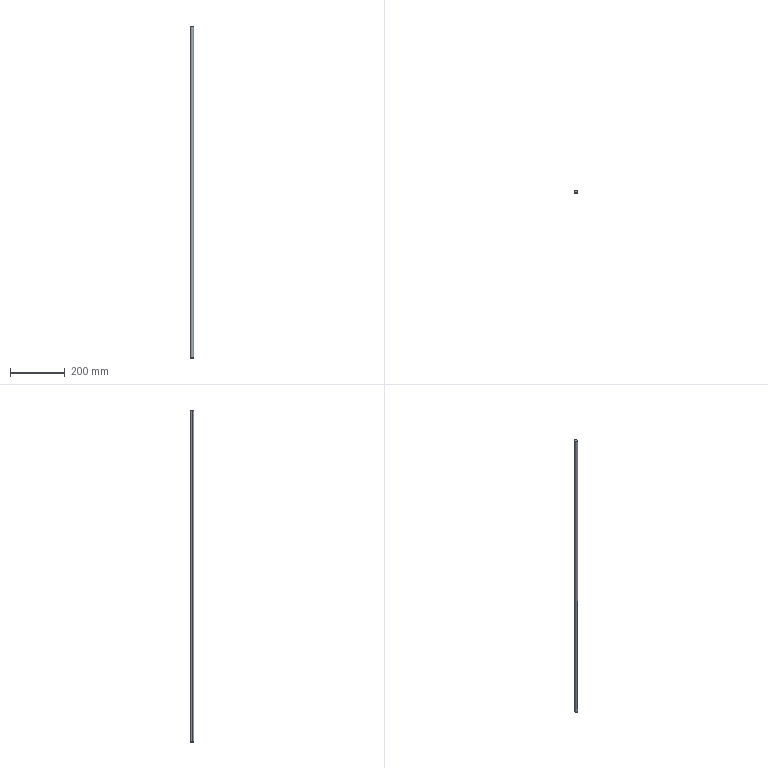Part | STEP file | SOP hanger | 1 solid | 8 faces | box 12 x 12 x 1210 mm | volume 136812 mm3 | cone 4 | cylinder 2 | plane 2 | commonest cylinder face diameters 12 x2
STEP:
#1=CARTESIAN_POINT('',(0.,0.,0.));
#2=DIRECTION('',(0.,0.,1.));
#3=DIRECTION('',(1.,0.,0.));
#4=AXIS2_PLACEMENT_3D('',#1,#2,#3);
#5=CARTESIAN_POINT('',(-6.,0.,1209.));
#6=VERTEX_POINT('',#5);
#7=CARTESIAN_POINT('',(6.,0.,1209.));
#8=VERTEX_POINT('',#7);
#9=CARTESIAN_POINT('',(0.,0.,1209.));
#10=DIRECTION('',(0.,0.,-1.));
#11=DIRECTION('',(-1.,0.,0.));
#12=AXIS2_PLACEMENT_3D('',#9,#10,#11);
#13=CIRCLE('',#12,6.);
#14=CARTESIAN_POINT('',(0.,0.,1210.));
#15=DIRECTION('',(0.,0.,-1.));
#16=DIRECTION('',(-1.,0.,0.));
#17=AXIS2_PLACEMENT_3D('',#14,#15,#16);
#18=CYLINDRICAL_SURFACE('',#17,6.);
#19=CARTESIAN_POINT('',(0.,1.));
#20=DIRECTION('',(1.,0.));
#21=VECTOR('',#20,1.);
#22=LINE('',#19,#21);
#23=(GEOMETRIC_REPRESENTATION_CONTEXT(2)PARAMETRIC_REPRESENTATION_CONTEXT()REPRESENTATION_CONTEXT('',''));
#24=DEFINITIONAL_REPRESENTATION('',(#22),#23);
#25=PCURVE('',#18,#24);
#26=CARTESIAN_POINT('',(0.,0.,1209.));
#27=DIRECTION('',(0.,0.,-1.));
#28=DIRECTION('',(-1.,0.,0.));
#29=AXIS2_PLACEMENT_3D('',#26,#27,#28);
#30=CONICAL_SURFACE('',#29,6.,0.7854);
#31=CARTESIAN_POINT('',(0.,0.));
#32=DIRECTION('',(1.,0.));
#33=VECTOR('',#32,1.);
#34=LINE('',#31,#33);
#35=(GEOMETRIC_REPRESENTATION_CONTEXT(2)PARAMETRIC_REPRESENTATION_CONTEXT()REPRESENTATION_CONTEXT('',''));
#36=DEFINITIONAL_REPRESENTATION('',(#34),#35);
#37=PCURVE('',#30,#36);
#38=SURFACE_CURVE('',#13,(#25,#37),.PCURVE_S1.);
#39=EDGE_CURVE('',#6,#8,#38,.T.);
#40=ORIENTED_EDGE('',*,*,#39,.T.);
#41=CARTESIAN_POINT('',(6.,0.,1.));
#42=VERTEX_POINT('',#41);
#43=CARTESIAN_POINT('',(6.,0.,1210.));
#44=DIRECTION('',(0.,0.,-1.));
#45=VECTOR('',#44,1.);
#46=LINE('',#43,#45);
#47=CARTESIAN_POINT('',(3.142,0.));
#48=DIRECTION('',(0.,1.));
#49=VECTOR('',#48,1.);
#50=LINE('',#47,#49);
#51=(GEOMETRIC_REPRESENTATION_CONTEXT(2)PARAMETRIC_REPRESENTATION_CONTEXT()REPRESENTATION_CONTEXT('',''));
#52=DEFINITIONAL_REPRESENTATION('',(#50),#51);
#53=PCURVE('',#18,#52);
#54=CARTESIAN_POINT('',(0.,0.,1210.));
#55=DIRECTION('',(0.,0.,-1.));
#56=DIRECTION('',(-1.,0.,0.));
#57=AXIS2_PLACEMENT_3D('',#54,#55,#56);
#58=CYLINDRICAL_SURFACE('',#57,6.);
#59=CARTESIAN_POINT('',(3.142,0.));
#60=DIRECTION('',(0.,1.));
#61=VECTOR('',#60,1.);
#62=LINE('',#59,#61);
#63=(GEOMETRIC_REPRESENTATION_CONTEXT(2)PARAMETRIC_REPRESENTATION_CONTEXT()REPRESENTATION_CONTEXT('',''));
#64=DEFINITIONAL_REPRESENTATION('',(#62),#63);
#65=PCURVE('',#58,#64);
#66=SURFACE_CURVE('',#46,(#53,#65),.PCURVE_S1.);
#67=EDGE_CURVE('',#8,#42,#66,.T.);
#68=ORIENTED_EDGE('',*,*,#67,.T.);
#69=CARTESIAN_POINT('',(-6.,0.,1.));
#70=VERTEX_POINT('',#69);
#71=CARTESIAN_POINT('',(0.,0.,1.));
#72=DIRECTION('',(0.,0.,1.));
#73=DIRECTION('',(-1.,0.,0.));
#74=AXIS2_PLACEMENT_3D('',#71,#72,#73);
#75=CIRCLE('',#74,6.);
#76=CARTESIAN_POINT('',(6.283,1209.));
#77=DIRECTION('',(-1.,0.));
#78=VECTOR('',#77,1.);
#79=LINE('',#76,#78);
#80=(GEOMETRIC_REPRESENTATION_CONTEXT(2)PARAMETRIC_REPRESENTATION_CONTEXT()REPRESENTATION_CONTEXT('',''));
#81=DEFINITIONAL_REPRESENTATION('',(#79),#80);
#82=PCURVE('',#18,#81);
#83=CARTESIAN_POINT('',(0.,0.,1.));
#84=DIRECTION('',(0.,0.,1.));
#85=DIRECTION('',(1.,0.,0.));
#86=AXIS2_PLACEMENT_3D('',#83,#84,#85);
#87=CONICAL_SURFACE('',#86,6.,0.7854);
#88=CARTESIAN_POINT('',(-3.142,0.));
#89=DIRECTION('',(1.,0.));
#90=VECTOR('',#89,1.);
#91=LINE('',#88,#90);
#92=(GEOMETRIC_REPRESENTATION_CONTEXT(2)PARAMETRIC_REPRESENTATION_CONTEXT()REPRESENTATION_CONTEXT('',''));
#93=DEFINITIONAL_REPRESENTATION('',(#91),#92);
#94=PCURVE('',#87,#93);
#95=SURFACE_CURVE('',#75,(#82,#94),.PCURVE_S1.);
#96=EDGE_CURVE('',#42,#70,#95,.T.);
#97=ORIENTED_EDGE('',*,*,#96,.T.);
#98=CARTESIAN_POINT('',(-6.,0.,1210.));
#99=DIRECTION('',(0.,0.,-1.));
#100=VECTOR('',#99,1.);
#101=LINE('',#98,#100);
#102=CARTESIAN_POINT('',(0.,0.));
#103=DIRECTION('',(0.,1.));
#104=VECTOR('',#103,1.);
#105=LINE('',#102,#104);
#106=(GEOMETRIC_REPRESENTATION_CONTEXT(2)PARAMETRIC_REPRESENTATION_CONTEXT()REPRESENTATION_CONTEXT('',''));
#107=DEFINITIONAL_REPRESENTATION('',(#105),#106);
#108=PCURVE('',#18,#107);
#109=CARTESIAN_POINT('',(6.283,0.));
#110=DIRECTION('',(0.,1.));
#111=VECTOR('',#110,1.);
#112=LINE('',#109,#111);
#113=(GEOMETRIC_REPRESENTATION_CONTEXT(2)PARAMETRIC_REPRESENTATION_CONTEXT()REPRESENTATION_CONTEXT('',''));
#114=DEFINITIONAL_REPRESENTATION('',(#112),#113);
#115=PCURVE('',#58,#114);
#116=SURFACE_CURVE('',#101,(#108,#115),.PCURVE_S1.);
#117=EDGE_CURVE('',#6,#70,#116,.T.);
#118=ORIENTED_EDGE('',*,*,#117,.F.);
#119=EDGE_LOOP('',(#40,#68,#97,#118));
#120=FACE_BOUND('',#119,.T.);
#121=ADVANCED_FACE('',(#120),#18,.T.);
#122=CARTESIAN_POINT('',(5.,0.,0.));
#123=VERTEX_POINT('',#122);
#124=CARTESIAN_POINT('',(-5.,0.,0.));
#125=VERTEX_POINT('',#124);
#126=CARTESIAN_POINT('',(0.,0.,0.));
#127=DIRECTION('',(0.,0.,1.));
#128=DIRECTION('',(1.,0.,0.));
#129=AXIS2_PLACEMENT_3D('',#126,#127,#128);
#130=CIRCLE('',#129,5.);
#131=CARTESIAN_POINT('',(0.,-1.));
#132=DIRECTION('',(1.,0.));
#133=VECTOR('',#132,1.);
#134=LINE('',#131,#133);
#135=(GEOMETRIC_REPRESENTATION_CONTEXT(2)PARAMETRIC_REPRESENTATION_CONTEXT()REPRESENTATION_CONTEXT('',''));
#136=DEFINITIONAL_REPRESENTATION('',(#134),#135);
#137=PCURVE('',#87,#136);
#138=CARTESIAN_POINT('',(0.,0.,0.));
#139=DIRECTION('',(0.,0.,1.));
#140=DIRECTION('',(1.,0.,0.));
#141=AXIS2_PLACEMENT_3D('',#138,#139,#140);
#142=PLANE('',#141);
#143=CARTESIAN_POINT('',(0.,0.));
#144=DIRECTION('',(1.,0.));
#145=AXIS2_PLACEMENT_2D('',#143,#144);
#146=CIRCLE('',#145,5.);
#147=(GEOMETRIC_REPRESENTATION_CONTEXT(2)PARAMETRIC_REPRESENTATION_CONTEXT()REPRESENTATION_CONTEXT('',''));
#148=DEFINITIONAL_REPRESENTATION('',(#146),#147);
#149=PCURVE('',#142,#148);
#150=SURFACE_CURVE('',#130,(#137,#149),.PCURVE_S1.);
#151=EDGE_CURVE('',#123,#125,#150,.T.);
#152=ORIENTED_EDGE('',*,*,#151,.T.);
#153=CARTESIAN_POINT('',(-6.,0.,1.));
#154=DIRECTION('',(-0.7071,0.,0.7071));
#155=VECTOR('',#154,1.);
#156=LINE('',#153,#155);
#157=CARTESIAN_POINT('',(3.142,0.));
#158=DIRECTION('',(0.,1.));
#159=VECTOR('',#158,1.);
#160=LINE('',#157,#159);
#161=(GEOMETRIC_REPRESENTATION_CONTEXT(2)PARAMETRIC_REPRESENTATION_CONTEXT()REPRESENTATION_CONTEXT('',''));
#162=DEFINITIONAL_REPRESENTATION('',(#160),#161);
#163=PCURVE('',#87,#162);
#164=CARTESIAN_POINT('',(0.,0.,1.));
#165=DIRECTION('',(0.,0.,1.));
#166=DIRECTION('',(1.,0.,0.));
#167=AXIS2_PLACEMENT_3D('',#164,#165,#166);
#168=CONICAL_SURFACE('',#167,6.,0.7854);
#169=CARTESIAN_POINT('',(3.142,0.));
#170=DIRECTION('',(0.,1.));
#171=VECTOR('',#170,1.);
#172=LINE('',#169,#171);
#173=(GEOMETRIC_REPRESENTATION_CONTEXT(2)PARAMETRIC_REPRESENTATION_CONTEXT()REPRESENTATION_CONTEXT('',''));
#174=DEFINITIONAL_REPRESENTATION('',(#172),#173);
#175=PCURVE('',#168,#174);
#176=SURFACE_CURVE('',#156,(#163,#175),.PCURVE_S1.);
#177=EDGE_CURVE('',#125,#70,#176,.T.);
#178=ORIENTED_EDGE('',*,*,#177,.T.);
#179=ORIENTED_EDGE('',*,*,#96,.F.);
#180=CARTESIAN_POINT('',(6.,0.,1.));
#181=DIRECTION('',(0.7071,0.,0.7071));
#182=VECTOR('',#181,1.);
#183=LINE('',#180,#182);
#184=CARTESIAN_POINT('',(0.,0.));
#185=DIRECTION('',(0.,1.));
#186=VECTOR('',#185,1.);
#187=LINE('',#184,#186);
#188=(GEOMETRIC_REPRESENTATION_CONTEXT(2)PARAMETRIC_REPRESENTATION_CONTEXT()REPRESENTATION_CONTEXT('',''));
#189=DEFINITIONAL_REPRESENTATION('',(#187),#188);
#190=PCURVE('',#87,#189);
#191=CARTESIAN_POINT('',(6.283,0.));
#192=DIRECTION('',(0.,1.));
#193=VECTOR('',#192,1.);
#194=LINE('',#191,#193);
#195=(GEOMETRIC_REPRESENTATION_CONTEXT(2)PARAMETRIC_REPRESENTATION_CONTEXT()REPRESENTATION_CONTEXT('',''));
#196=DEFINITIONAL_REPRESENTATION('',(#194),#195);
#197=PCURVE('',#168,#196);
#198=SURFACE_CURVE('',#183,(#190,#197),.PCURVE_S1.);
#199=EDGE_CURVE('',#123,#42,#198,.T.);
#200=ORIENTED_EDGE('',*,*,#199,.F.);
#201=EDGE_LOOP('',(#152,#178,#179,#200));
#202=FACE_BOUND('',#201,.T.);
#203=ADVANCED_FACE('',(#202),#87,.T.);
#204=CARTESIAN_POINT('',(-5.,0.,1210.));
#205=VERTEX_POINT('',#204);
#206=CARTESIAN_POINT('',(5.,0.,1210.));
#207=VERTEX_POINT('',#206);
#208=CARTESIAN_POINT('',(0.,0.,1210.));
#209=DIRECTION('',(0.,0.,-1.));
#210=DIRECTION('',(-1.,0.,0.));
#211=AXIS2_PLACEMENT_3D('',#208,#209,#210);
#212=CIRCLE('',#211,5.);
#213=CARTESIAN_POINT('',(0.,-1.));
#214=DIRECTION('',(1.,0.));
#215=VECTOR('',#214,1.);
#216=LINE('',#213,#215);
#217=(GEOMETRIC_REPRESENTATION_CONTEXT(2)PARAMETRIC_REPRESENTATION_CONTEXT()REPRESENTATION_CONTEXT('',''));
#218=DEFINITIONAL_REPRESENTATION('',(#216),#217);
#219=PCURVE('',#30,#218);
#220=CARTESIAN_POINT('',(0.,0.,1210.));
#221=DIRECTION('',(0.,0.,1.));
#222=DIRECTION('',(1.,0.,0.));
#223=AXIS2_PLACEMENT_3D('',#220,#221,#222);
#224=PLANE('',#223);
#225=CARTESIAN_POINT('',(-5.,0.));
#226=CARTESIAN_POINT('',(-5.,8.66));
#227=CARTESIAN_POINT('',(2.5,4.33));
#228=CARTESIAN_POINT('',(10.,0.));
#229=CARTESIAN_POINT('',(2.5,-4.33));
#230=CARTESIAN_POINT('',(-5.,-8.66));
#231=CARTESIAN_POINT('',(-5.,0.));
#232=(BOUNDED_CURVE()B_SPLINE_CURVE(2,(#225,#226,#227,#228,#229,#230,#231),.UNSPECIFIED.,.T.,.F.)B_SPLINE_CURVE_WITH_KNOTS((1,2,2,2,2,1),(-2.094,0.,2.094,4.189,6.283,8.378),.UNSPECIFIED.)CURVE()GEOMETRIC_REPRESENTATION_ITEM()RATIONAL_B_SPLINE_CURVE((1.,0.5,1.,0.5,1.,0.5,1.))REPRESENTATION_ITEM(''));
#233=(GEOMETRIC_REPRESENTATION_CONTEXT(2)PARAMETRIC_REPRESENTATION_CONTEXT()REPRESENTATION_CONTEXT('',''));
#234=DEFINITIONAL_REPRESENTATION('',(#232),#233);
#235=PCURVE('',#224,#234);
#236=SURFACE_CURVE('',#212,(#219,#235),.PCURVE_S1.);
#237=EDGE_CURVE('',#205,#207,#236,.T.);
#238=ORIENTED_EDGE('',*,*,#237,.T.);
#239=CARTESIAN_POINT('',(6.,0.,1209.));
#240=DIRECTION('',(0.7071,0.,-0.7071));
#241=VECTOR('',#240,1.);
#242=LINE('',#239,#241);
#243=CARTESIAN_POINT('',(3.142,0.));
#244=DIRECTION('',(0.,1.));
#245=VECTOR('',#244,1.);
#246=LINE('',#243,#245);
#247=(GEOMETRIC_REPRESENTATION_CONTEXT(2)PARAMETRIC_REPRESENTATION_CONTEXT()REPRESENTATION_CONTEXT('',''));
#248=DEFINITIONAL_REPRESENTATION('',(#246),#247);
#249=PCURVE('',#30,#248);
#250=CARTESIAN_POINT('',(0.,0.,1209.));
#251=DIRECTION('',(0.,0.,-1.));
#252=DIRECTION('',(-1.,0.,0.));
#253=AXIS2_PLACEMENT_3D('',#250,#251,#252);
#254=CONICAL_SURFACE('',#253,6.,0.7854);
#255=CARTESIAN_POINT('',(3.142,0.));
#256=DIRECTION('',(0.,1.));
#257=VECTOR('',#256,1.);
#258=LINE('',#255,#257);
#259=(GEOMETRIC_REPRESENTATION_CONTEXT(2)PARAMETRIC_REPRESENTATION_CONTEXT()REPRESENTATION_CONTEXT('',''));
#260=DEFINITIONAL_REPRESENTATION('',(#258),#259);
#261=PCURVE('',#254,#260);
#262=SURFACE_CURVE('',#242,(#249,#261),.PCURVE_S1.);
#263=EDGE_CURVE('',#207,#8,#262,.T.);
#264=ORIENTED_EDGE('',*,*,#263,.T.);
#265=ORIENTED_EDGE('',*,*,#39,.F.);
#266=CARTESIAN_POINT('',(-6.,0.,1209.));
#267=DIRECTION('',(-0.7071,0.,-0.7071));
#268=VECTOR('',#267,1.);
#269=LINE('',#266,#268);
#270=CARTESIAN_POINT('',(0.,0.));
#271=DIRECTION('',(0.,1.));
#272=VECTOR('',#271,1.);
#273=LINE('',#270,#272);
#274=(GEOMETRIC_REPRESENTATION_CONTEXT(2)PARAMETRIC_REPRESENTATION_CONTEXT()REPRESENTATION_CONTEXT('',''));
#275=DEFINITIONAL_REPRESENTATION('',(#273),#274);
#276=PCURVE('',#30,#275);
#277=CARTESIAN_POINT('',(6.283,0.));
#278=DIRECTION('',(0.,1.));
#279=VECTOR('',#278,1.);
#280=LINE('',#277,#279);
#281=(GEOMETRIC_REPRESENTATION_CONTEXT(2)PARAMETRIC_REPRESENTATION_CONTEXT()REPRESENTATION_CONTEXT('',''));
#282=DEFINITIONAL_REPRESENTATION('',(#280),#281);
#283=PCURVE('',#254,#282);
#284=SURFACE_CURVE('',#269,(#276,#283),.PCURVE_S1.);
#285=EDGE_CURVE('',#205,#6,#284,.T.);
#286=ORIENTED_EDGE('',*,*,#285,.F.);
#287=EDGE_LOOP('',(#238,#264,#265,#286));
#288=FACE_BOUND('',#287,.T.);
#289=ADVANCED_FACE('',(#288),#30,.T.);
#290=ORIENTED_EDGE('',*,*,#67,.F.);
#291=CARTESIAN_POINT('',(0.,0.,1209.));
#292=DIRECTION('',(0.,0.,-1.));
#293=DIRECTION('',(-1.,0.,0.));
#294=AXIS2_PLACEMENT_3D('',#291,#292,#293);
#295=CIRCLE('',#294,6.);
#296=CARTESIAN_POINT('',(0.,1.));
#297=DIRECTION('',(1.,0.));
#298=VECTOR('',#297,1.);
#299=LINE('',#296,#298);
#300=(GEOMETRIC_REPRESENTATION_CONTEXT(2)PARAMETRIC_REPRESENTATION_CONTEXT()REPRESENTATION_CONTEXT('',''));
#301=DEFINITIONAL_REPRESENTATION('',(#299),#300);
#302=PCURVE('',#58,#301);
#303=CARTESIAN_POINT('',(0.,0.));
#304=DIRECTION('',(1.,0.));
#305=VECTOR('',#304,1.);
#306=LINE('',#303,#305);
#307=(GEOMETRIC_REPRESENTATION_CONTEXT(2)PARAMETRIC_REPRESENTATION_CONTEXT()REPRESENTATION_CONTEXT('',''));
#308=DEFINITIONAL_REPRESENTATION('',(#306),#307);
#309=PCURVE('',#254,#308);
#310=SURFACE_CURVE('',#295,(#302,#309),.PCURVE_S1.);
#311=EDGE_CURVE('',#8,#6,#310,.T.);
#312=ORIENTED_EDGE('',*,*,#311,.T.);
#313=ORIENTED_EDGE('',*,*,#117,.T.);
#314=CARTESIAN_POINT('',(0.,0.,1.));
#315=DIRECTION('',(0.,0.,1.));
#316=DIRECTION('',(-1.,0.,0.));
#317=AXIS2_PLACEMENT_3D('',#314,#315,#316);
#318=CIRCLE('',#317,6.);
#319=CARTESIAN_POINT('',(6.283,1209.));
#320=DIRECTION('',(-1.,0.));
#321=VECTOR('',#320,1.);
#322=LINE('',#319,#321);
#323=(GEOMETRIC_REPRESENTATION_CONTEXT(2)PARAMETRIC_REPRESENTATION_CONTEXT()REPRESENTATION_CONTEXT('',''));
#324=DEFINITIONAL_REPRESENTATION('',(#322),#323);
#325=PCURVE('',#58,#324);
#326=CARTESIAN_POINT('',(3.142,0.));
#327=DIRECTION('',(1.,0.));
#328=VECTOR('',#327,1.);
#329=LINE('',#326,#328);
#330=(GEOMETRIC_REPRESENTATION_CONTEXT(2)PARAMETRIC_REPRESENTATION_CONTEXT()REPRESENTATION_CONTEXT('',''));
#331=DEFINITIONAL_REPRESENTATION('',(#329),#330);
#332=PCURVE('',#168,#331);
#333=SURFACE_CURVE('',#318,(#325,#332),.PCURVE_S1.);
#334=EDGE_CURVE('',#70,#42,#333,.T.);
#335=ORIENTED_EDGE('',*,*,#334,.T.);
#336=EDGE_LOOP('',(#290,#312,#313,#335));
#337=FACE_BOUND('',#336,.T.);
#338=ADVANCED_FACE('',(#337),#58,.T.);
#339=ORIENTED_EDGE('',*,*,#177,.F.);
#340=CARTESIAN_POINT('',(0.,0.,0.));
#341=DIRECTION('',(0.,0.,1.));
#342=DIRECTION('',(1.,0.,0.));
#343=AXIS2_PLACEMENT_3D('',#340,#341,#342);
#344=CIRCLE('',#343,5.);
#345=CARTESIAN_POINT('',(0.,-1.));
#346=DIRECTION('',(1.,0.));
#347=VECTOR('',#346,1.);
#348=LINE('',#345,#347);
#349=(GEOMETRIC_REPRESENTATION_CONTEXT(2)PARAMETRIC_REPRESENTATION_CONTEXT()REPRESENTATION_CONTEXT('',''));
#350=DEFINITIONAL_REPRESENTATION('',(#348),#349);
#351=PCURVE('',#168,#350);
#352=CARTESIAN_POINT('',(0.,0.));
#353=DIRECTION('',(1.,0.));
#354=AXIS2_PLACEMENT_2D('',#352,#353);
#355=CIRCLE('',#354,5.);
#356=(GEOMETRIC_REPRESENTATION_CONTEXT(2)PARAMETRIC_REPRESENTATION_CONTEXT()REPRESENTATION_CONTEXT('',''));
#357=DEFINITIONAL_REPRESENTATION('',(#355),#356);
#358=PCURVE('',#142,#357);
#359=SURFACE_CURVE('',#344,(#351,#358),.PCURVE_S1.);
#360=EDGE_CURVE('',#125,#123,#359,.T.);
#361=ORIENTED_EDGE('',*,*,#360,.T.);
#362=ORIENTED_EDGE('',*,*,#199,.T.);
#363=ORIENTED_EDGE('',*,*,#334,.F.);
#364=EDGE_LOOP('',(#339,#361,#362,#363));
#365=FACE_BOUND('',#364,.T.);
#366=ADVANCED_FACE('',(#365),#168,.T.);
#367=ORIENTED_EDGE('',*,*,#263,.F.);
#368=CARTESIAN_POINT('',(0.,0.,1210.));
#369=DIRECTION('',(0.,0.,-1.));
#370=DIRECTION('',(-1.,0.,0.));
#371=AXIS2_PLACEMENT_3D('',#368,#369,#370);
#372=CIRCLE('',#371,5.);
#373=CARTESIAN_POINT('',(0.,-1.));
#374=DIRECTION('',(1.,0.));
#375=VECTOR('',#374,1.);
#376=LINE('',#373,#375);
#377=(GEOMETRIC_REPRESENTATION_CONTEXT(2)PARAMETRIC_REPRESENTATION_CONTEXT()REPRESENTATION_CONTEXT('',''));
#378=DEFINITIONAL_REPRESENTATION('',(#376),#377);
#379=PCURVE('',#254,#378);
#380=CARTESIAN_POINT('',(-5.,0.));
#381=CARTESIAN_POINT('',(-5.,8.66));
#382=CARTESIAN_POINT('',(2.5,4.33));
#383=CARTESIAN_POINT('',(10.,0.));
#384=CARTESIAN_POINT('',(2.5,-4.33));
#385=CARTESIAN_POINT('',(-5.,-8.66));
#386=CARTESIAN_POINT('',(-5.,0.));
#387=(BOUNDED_CURVE()B_SPLINE_CURVE(2,(#380,#381,#382,#383,#384,#385,#386),.UNSPECIFIED.,.T.,.F.)B_SPLINE_CURVE_WITH_KNOTS((1,2,2,2,2,1),(-2.094,0.,2.094,4.189,6.283,8.378),.UNSPECIFIED.)CURVE()GEOMETRIC_REPRESENTATION_ITEM()RATIONAL_B_SPLINE_CURVE((1.,0.5,1.,0.5,1.,0.5,1.))REPRESENTATION_ITEM(''));
#388=(GEOMETRIC_REPRESENTATION_CONTEXT(2)PARAMETRIC_REPRESENTATION_CONTEXT()REPRESENTATION_CONTEXT('',''));
#389=DEFINITIONAL_REPRESENTATION('',(#387),#388);
#390=PCURVE('',#224,#389);
#391=SURFACE_CURVE('',#372,(#379,#390),.PCURVE_S1.);
#392=EDGE_CURVE('',#207,#205,#391,.T.);
#393=ORIENTED_EDGE('',*,*,#392,.T.);
#394=ORIENTED_EDGE('',*,*,#285,.T.);
#395=ORIENTED_EDGE('',*,*,#311,.F.);
#396=EDGE_LOOP('',(#367,#393,#394,#395));
#397=FACE_BOUND('',#396,.T.);
#398=ADVANCED_FACE('',(#397),#254,.T.);
#399=ORIENTED_EDGE('',*,*,#151,.F.);
#400=ORIENTED_EDGE('',*,*,#360,.F.);
#401=EDGE_LOOP('',(#399,#400));
#402=FACE_BOUND('',#401,.T.);
#403=ADVANCED_FACE('',(#402),#142,.F.);
#404=ORIENTED_EDGE('',*,*,#237,.F.);
#405=ORIENTED_EDGE('',*,*,#392,.F.);
#406=EDGE_LOOP('',(#404,#405));
#407=FACE_BOUND('',#406,.T.);
#408=ADVANCED_FACE('',(#407),#224,.T.);
#409=CLOSED_SHELL('',(#121,#203,#289,#338,#366,#398,#403,#408));
#410=MANIFOLD_SOLID_BREP('',#409);
#411=(LENGTH_UNIT()NAMED_UNIT(*)SI_UNIT(.MILLI.,.METRE.));
#412=UNCERTAINTY_MEASURE_WITH_UNIT(LENGTH_MEASURE(0.0000001),#411,'','');
#413=(NAMED_UNIT(*)PLANE_ANGLE_UNIT()SI_UNIT($,.RADIAN.));
#414=(NAMED_UNIT(*)SI_UNIT($,.STERADIAN.)SOLID_ANGLE_UNIT());
#415=(GEOMETRIC_REPRESENTATION_CONTEXT(3)GLOBAL_UNCERTAINTY_ASSIGNED_CONTEXT((#412))GLOBAL_UNIT_ASSIGNED_CONTEXT((#411,#413,#414))REPRESENTATION_CONTEXT('',''));
#416=ADVANCED_BREP_SHAPE_REPRESENTATION('',(#4,#410),#415);